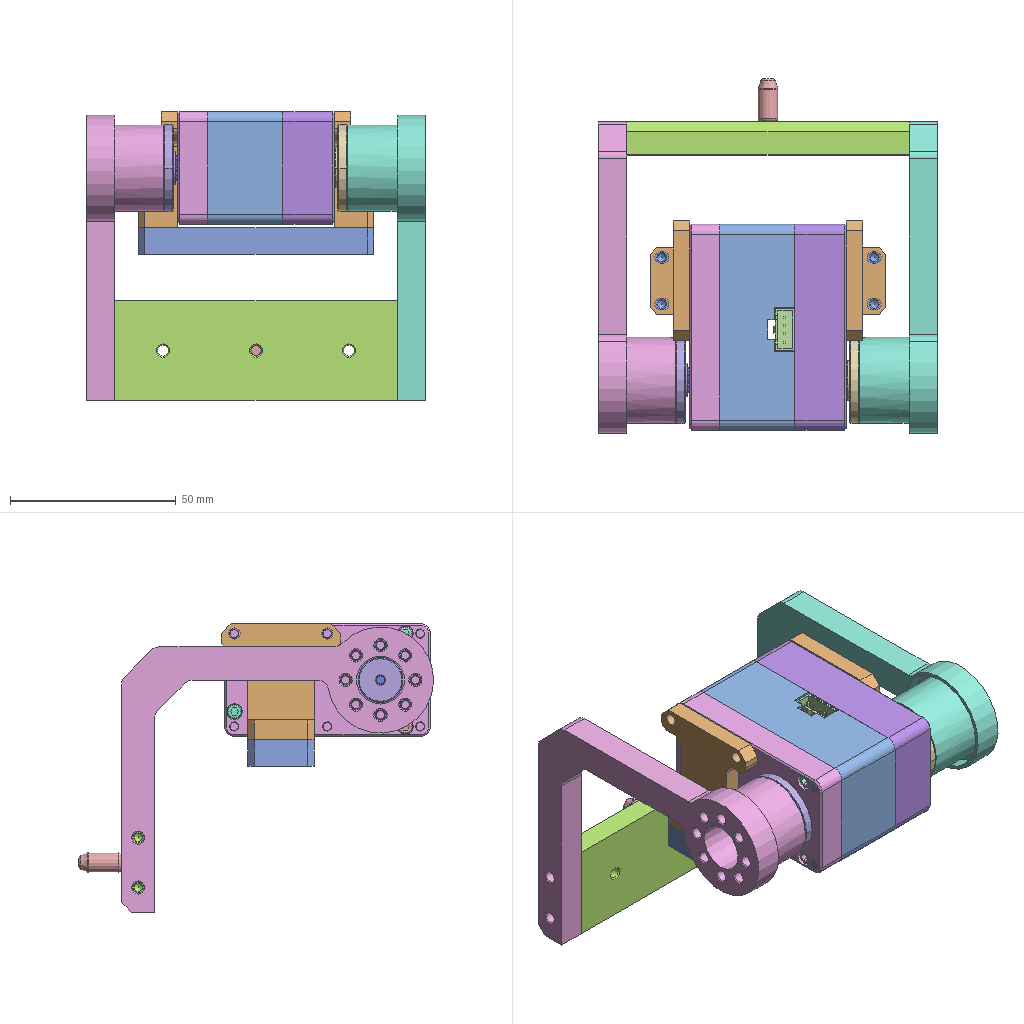Assembly | NX | 7 different items | 8 placed | box 102 x 107 x 87 mm
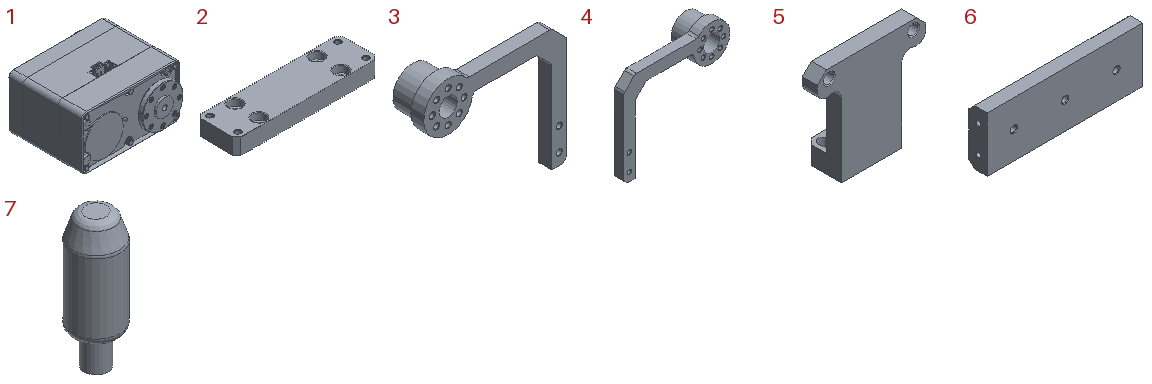Parts list (item | quantity | size | volume | features):
1 | x1 | - | 1762 mm3 | features BREP 21
2 | x1 | 71 x 20 x 8 mm | 10535 mm3 | features CBORE_HOLE 4, DATUM_CSYS 4, LINKED_CURVE 4, SIMPLE HOLE 4, SYMBOLIC_THREAD 4, SKETCH 3, HOLE PACKAGE 2, CHAMFER 1, EXTRUDE 1, LINKED_FACE 1
3 | x1 | 93.991 x 23.3 x 85.991 mm | 20704 mm3 | features DATUM_CSYS 12, SKETCH 11, SIMPLE HOLE 10, HOLE PACKAGE 9, EXTRACT_FACE 8, Instance Feature 7, CHAMFER 3, BLEND 2, CPROJ 1, EXTRUDE 1, OFFSET_REGION 1, Pattern Feature 1, SWP104 1
4 | x1 | 93.991 x 23.1 x 85.991 mm | 19432 mm3 | features DATUM_CSYS 12, SKETCH 11, SIMPLE HOLE 10, HOLE PACKAGE 9, EXTRACT_FACE 8, Instance Feature 7, BLEND 2, CHAMFER 2, CPROJ 1, DATUM_AXIS 1, EXTRUDE 1, LINKED_FACE 1, OFFSET_REGION 1, Pattern Feature 1, SWP104 1
5 | x2 | 36 x 12 x 35 mm | 4656 mm3 | features DATUM_CSYS 5, SKETCH 4, EXTRUDE 3, CHAMFER 2, OFFSET_REGION 2, SIMPLE HOLE 2, BLEND 1, HOLE PACKAGE 1
6 | x1 | 85 x 10 x 30 mm | 24243 mm3 | features SIMPLE HOLE 7, SYMBOLIC_THREAD 7, DATUM_CSYS 5, SKETCH 4, HOLE PACKAGE 3, OFFSET_REGION 2, CHAMFER 1, EXTRUDE 1, LINKED_FACE 1
7 | x1 | 6 x 6 x 17 mm | 365.792 mm3 | features DATUM_CSYS 2, BLEND 1, SKETCH 1, SWP104 1
Mates (type | each side: item.copy, entity, surface, feature):
Touch | 7.1 face cylinder Revolve(1) | 6.1 face cylinder M4 x 0.7 Threaded Hole(5)
Distance | 7.1 face plane Revolve(1) | 6.1 face plane Extrude(2)